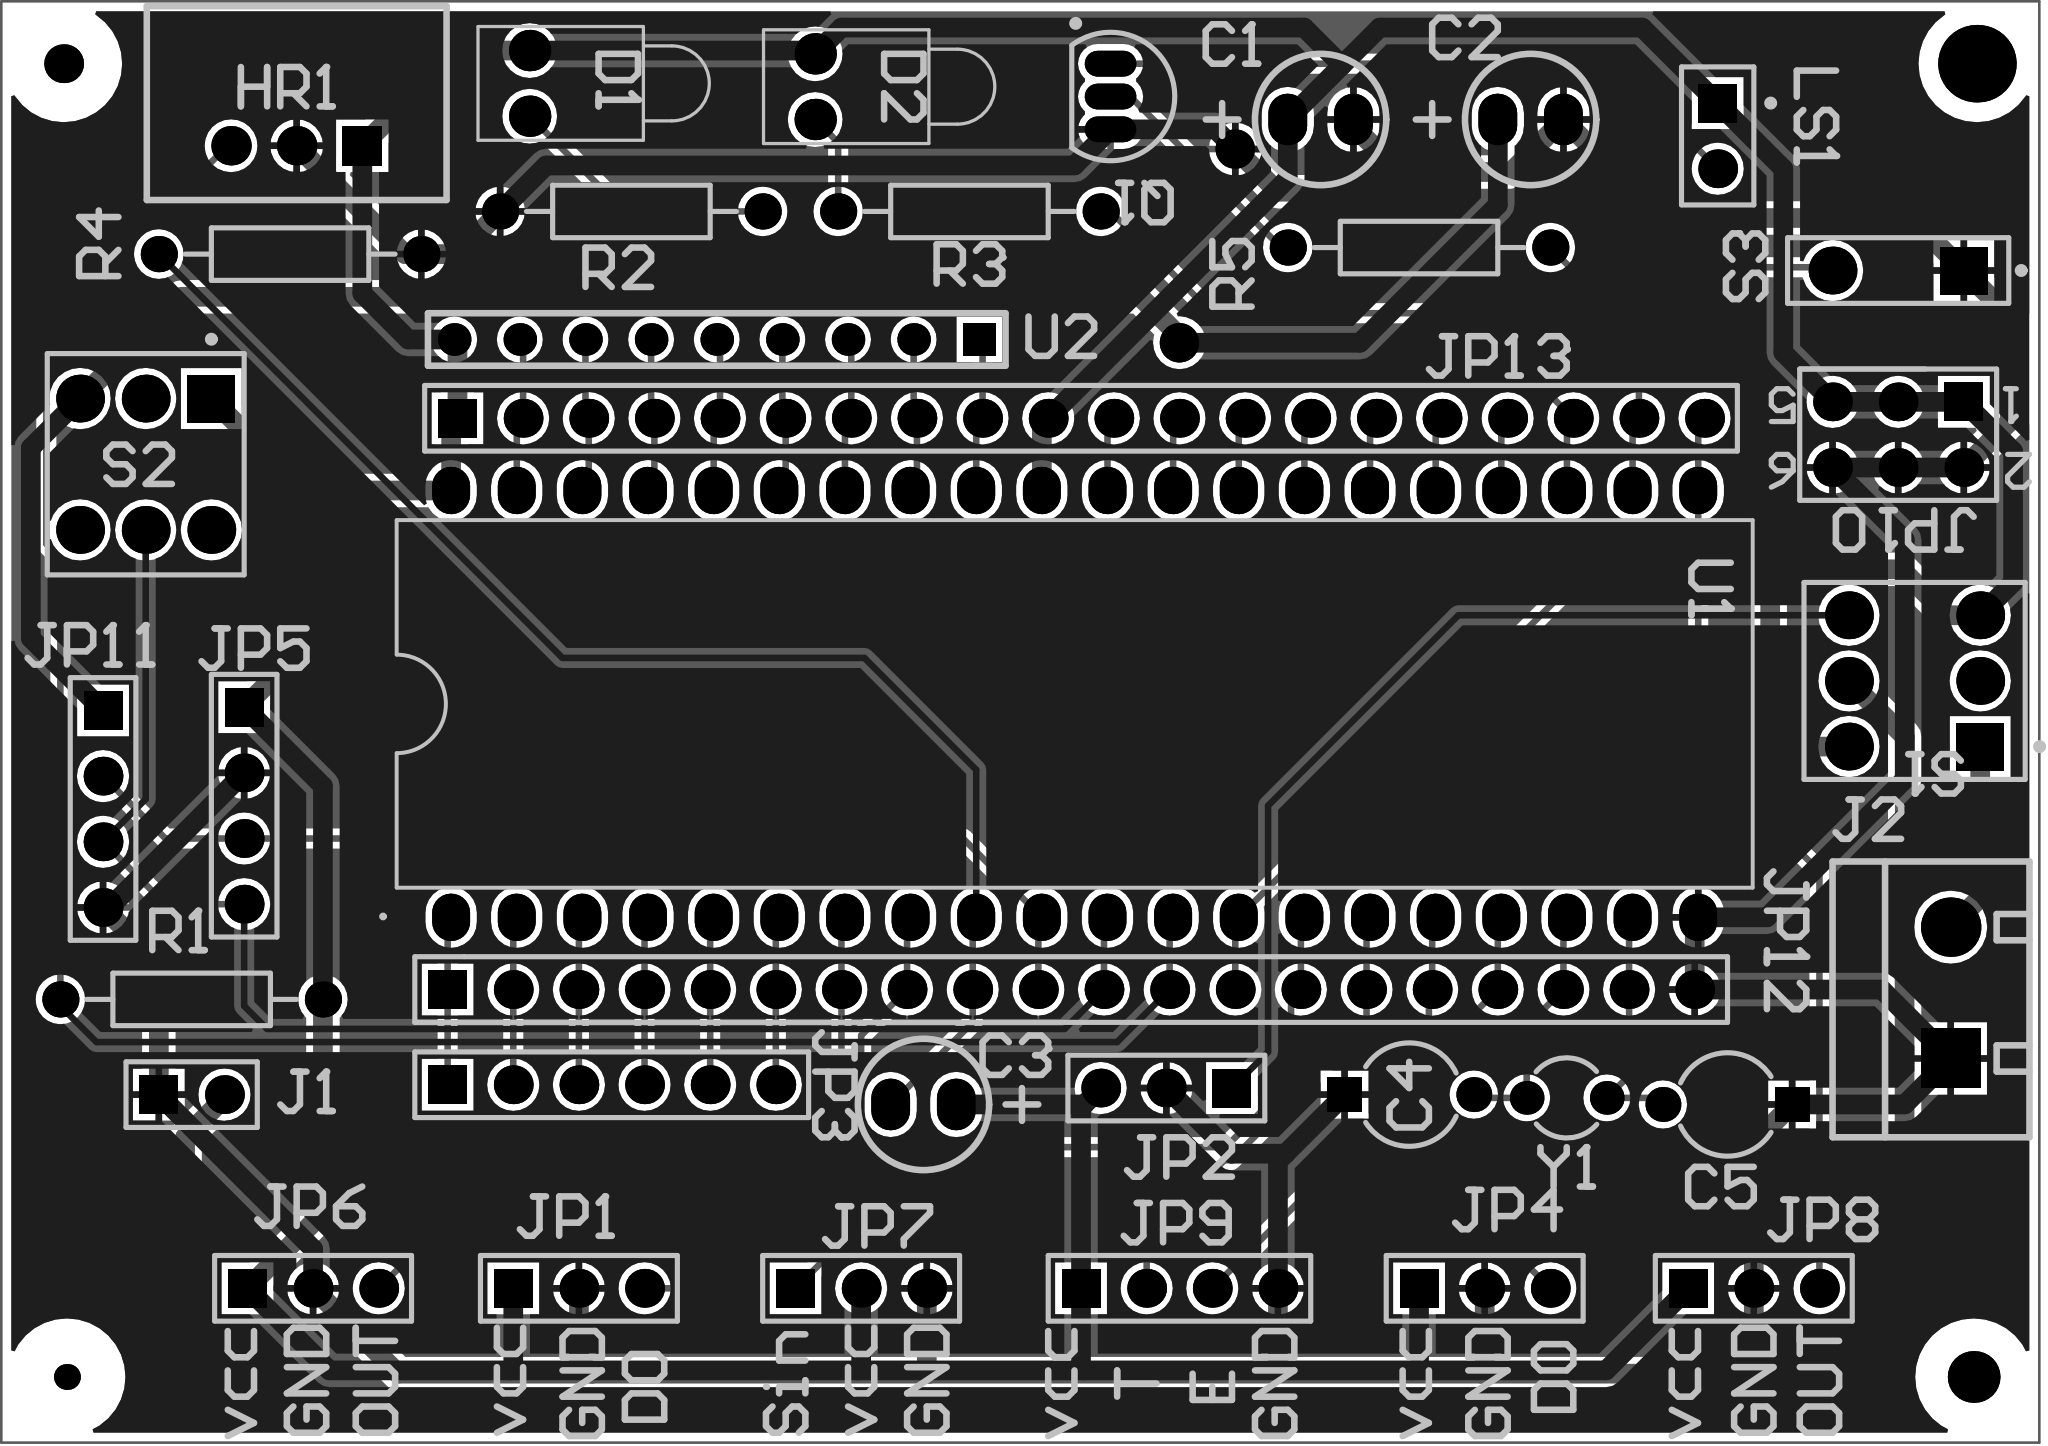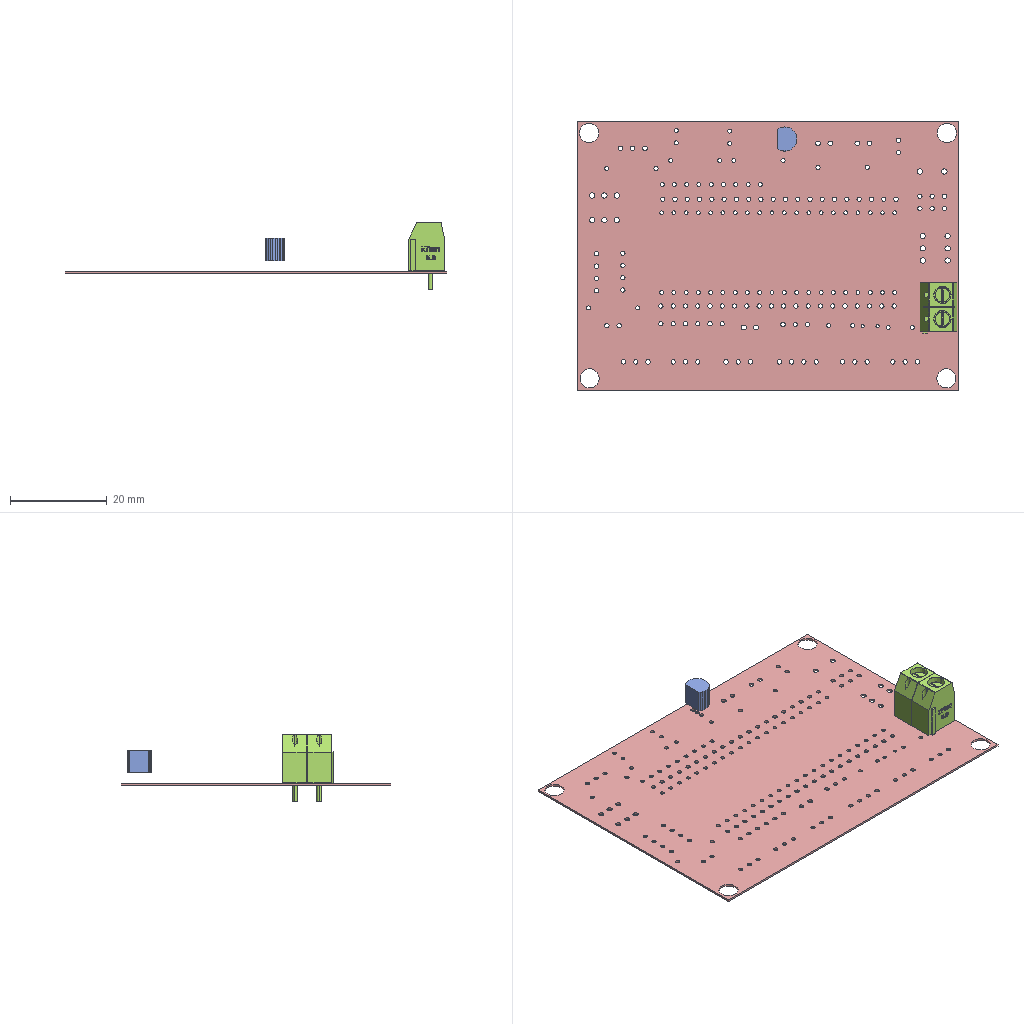Circuit board layout | Altium Designer | box 78.9 x 55.8 x 13.8 mm
Layer stack:
# Altium Designer layer stack of  (unit mm; dielectric type: 0 none, 1 core, 2 prepreg, 3 surface material)
index,name,kind,layer,copper_thickness_mm,dielectric_type,dielectric_thickness_mm,dielectric_material,dielectric_constant
0,Top Paste,other,,,,,,
1,Top Overlay,other,,,,,,
2,Top Solder,dielectric,,,3,0.0102,Solder Resist,3.5
3,Top Layer,copper,Top Layer,0.0356,,,,
4,Dielectric 1,dielectric,,,0,0.32,FR-4,4.8
5,Bottom Layer,copper,Bottom Layer,0.0356,,,,
6,Bottom Solder,dielectric,,,3,0.0102,Solder Resist,3.5
7,Bottom Overlay,other,,,,,,
8,Bottom Paste,other,,,,,,
# drill layer pairs: low layer,high layer
drill_pair,Top Layer,Bottom Layer
Part placement:
Designator,Comment,Layer,Footprint,Center-X(mm),Center-Y(mm),Rotation
Y1,11.059,TopLayer,R38,85.979,38.608,270
U2,Resistor network,TopLayer,paizu,53.086,67.945,180
U1,STC89C52RC,TopLayer,STC89C52RC,66.937,53.848,360
S3,SW-PB,TopLayer,SPST-2,98.806,70.612,180
S2,SW-DPDT,TopLayer,DPDT-6,30.988,63.119,270
S1,SW-DPDT,TopLayer,DPDT-6,99.441,54.737,180
R5,1K,TopLayer,AXIAL-0.4,80.264,71.501,180
R4,10K,TopLayer,AXIAL-0.4,36.576,71.247,180
R3,1K,TopLayer,AXIAL-0.4,62.865,72.898,360
R2,1K,TopLayer,AXIAL-0.4,49.784,72.898,180
R1,10K,TopLayer,AXIAL-0.4,32.766,42.418,180
Q1,2N3906,TopLayer,TO-92A,68.326,77.343,180
LS1,Bell,TopLayer,PIN2,91.821,75.819,270
JP13,Header 20,TopLayer,HDR1X20,67.183,64.897,360
JP12,Header 20,TopLayer,HDR1X20,66.802,42.799,360
JP11,Download interface,TopLayer,HDR1X4,29.337,49.784,270
JP10,Header 3X2,TopLayer,HDR2X3,98.806,64.262,180
JP9,Ultrasonic module,TopLayer,HDR1X4,70.993,31.242,360
JP8,Left obstacle avoidance,TopLayer,HDR1X3,93.218,31.242,360
JP7,Servo module,TopLayer,HDR1X3,58.674,31.242,360
JP6,Right obstacle avoidance,TopLayer,HDR1X3,37.465,31.242,360
JP5,Bluetooth module,TopLayer,HDR1X4,34.798,49.911,270
JP4,Left line tracking,TopLayer,HDR1X3,82.804,31.242,360
JP3,L298N control,TopLayer,HDR1X6,49.022,39.116,360
JP2,L298N power,TopLayer,HDR1X3,70.485,38.989,180
JP1,Right line tracking,TopLayer,HDR1X3,47.752,31.242,360
J2,KF301-2P,TopLayer,KF301-5.0-2P,100.838,42.672,90
J1,Header 2,TopLayer,HDR1X2,32.766,38.735,360
HR1,HR,TopLayer,SIP3,36.83,75.439,180
D2,Mode indicator LED,TopLayer,LED-1,56.896,77.724,360
D1,Power,TopLayer,LED-1,45.847,77.851,360
C5,22PF,TopLayer,CAPR5-4X5,92.202,38.354,180
C4,22PF,TopLayer,CAPR5-4X5,79.883,38.735,0
C3,10UF,TopLayer,DR,61.087,38.354,180
C2,470UF,TopLayer,DR,84.582,76.454,0
C1,470UF,TopLayer,DR,76.454,76.454,0
Pad and via stacks:
# Altium Designer via and pad stacks of  (unit mm). Each distinct definition once, with the count of objects using it.
# via: kind,start_layer,end_layer,hole_mm,diameter_mm,mode(0 simple;1 top-mid-bottom;2 full stack),diameter_per_layer,count,example_net
# pad: kind,layer,hole_mm,hole_type(0 round;1 square;2 slot),plating,top_size,top_shape(1 round;2 rect;3 octagon;9 rounded rect),mid_size,bottom_size,mode,footprint,size_per_layer,count,example
pad,Multi-Layer,4,0,plated,1.5x1.5,1,1.5x1.5,1.5x1.5,0,,,1,3
pad,Multi-Layer,4,0,plated,1x1,1,1x1,1x1,0,,,1,2
pad,Multi-Layer,4,0,plated,2x2,1,2x2,2x2,0,,,1,1
pad,Multi-Layer,4,0,plated,3x3,1,3x3,3x3,0,,,1,0
pad,Multi-Layer,0.9,0,plated,1.5x1.5,1,1.5x1.5,1.5x1.5,0,HDR1X4,,9,JP5.4
pad,Multi-Layer,0.9,0,plated,1.5x1.5,2,1.5x1.5,1.5x1.5,0,HDR1X4,,3,JP5.1
pad,Multi-Layer,1,0,plated,1.5x2,1,1.5x2,1.5x2,0,DR,,6,C3.1
pad,Multi-Layer,1.1,0,plated,1.85x1.85,1,1.85x1.85,1.85x1.85,0,DPDT-6,,10,S2.4
pad,Multi-Layer,1.1,0,plated,1.85x1.85,2,1.85x1.85,1.85x1.85,0,DPDT-6,,2,S2.1
pad,Multi-Layer,0.9,0,plated,1.5x1.5,2,1.5x1.5,1.5x1.5,0,HDR1X2,,1,J1.1
pad,Multi-Layer,0.9,0,plated,1.5x1.5,1,1.5x1.5,1.5x1.5,0,HDR1X2,,1,J1.2
pad,Multi-Layer,0.9144,0,plated,1.524x1.524,1,1.524x1.524,1.524x1.524,0,SIP3,,2,HR1.3
pad,Multi-Layer,0.9144,0,plated,1.524x1.524,2,1.524x1.524,1.524x1.524,0,SIP3,,1,HR1.1
pad,Multi-Layer,0.9,0,plated,1.5x1.5,2,1.5x1.5,1.5x1.5,0,HDR1X3,,6,JP1.1
pad,Multi-Layer,0.9,0,plated,1.5x1.5,1,1.5x1.5,1.5x1.5,0,HDR1X3,,12,JP1.2
pad,Multi-Layer,0.85,0,plated,1.4x1.4,1,1.4x1.4,1.4x1.4,0,AXIAL-0.4,,10,R1.1
pad,Multi-Layer,0.9,0,plated,1.5x1.5,2,1.5x1.5,1.5x1.5,0,HDR1X6,,1,JP3.1
pad,Multi-Layer,0.9,0,plated,1.5x1.5,1,1.5x1.5,1.5x1.5,0,HDR1X6,,5,JP3.2
pad,Multi-Layer,1.2,0,plated,2.3x2.3,2,2.3x2.3,2.3x2.3,0,KF301-5.0-2P,,1,J2.1
pad,Multi-Layer,1.2,0,plated,2.3x2.3,1,2.3x2.3,2.3x2.3,0,KF301-5.0-2P,,1,J2.2
pad,Multi-Layer,0.9,0,plated,1.5x1.5,2,1.5x1.5,1.5x1.5,0,HDR2X3,,1,JP10.1
pad,Multi-Layer,0.9,0,plated,1.5x1.5,1,1.5x1.5,1.5x1.5,0,HDR2X3,,5,JP10.2
pad,Multi-Layer,0.8,0,plated,1.6x1.6,1,1.6x1.6,1.6x1.6,0,LED-1,,4,D1.1
pad,Multi-Layer,0.9,0,plated,1.5x1.5,2,1.5x1.5,1.5x1.5,0,HDR1X20,,2,JP13.1
pad,Multi-Layer,0.9,0,plated,1.5x1.5,1,1.5x1.5,1.5x1.5,0,HDR1X20,,38,JP13.2
pad,Multi-Layer,0.84,0,plated,1.26x1.26,2,1.26x1.26,1.26x1.26,0,paizu,,1,U2.1
pad,Multi-Layer,0.84,0,plated,1.26x1.26,1,1.26x1.26,1.26x1.26,0,paizu,,8,U2.2
pad,Multi-Layer,0.8,0,plated,1.467x1.833,1,1.467x1.833,1.467x1.833,0,STC89C52RC,,40,U1.21
pad,Multi-Layer,1.1,0,plated,1.85x1.85,2,1.85x1.85,1.85x1.85,0,SPST-2,,1,S3.1
pad,Multi-Layer,1.1,0,plated,1.85x1.85,1,1.85x1.85,1.85x1.85,0,SPST-2,,1,S3.2
pad,Multi-Layer,0.9,0,plated,1.5x1.5,2,1.5x1.5,1.5x1.5,0,PIN2,,1,LS1.1
pad,Multi-Layer,0.9,0,plated,1.5x1.5,1,1.5x1.5,1.5x1.5,0,PIN2,,1,LS1.2
pad,Multi-Layer,0.8,0,plated,1.35x1.35,1,1.35x1.35,1.35x1.35,0,CAPR5-4X5,,2,C4.2
pad,Multi-Layer,0.8,0,plated,1.35x1.35,2,1.35x1.35,1.35x1.35,0,CAPR5-4X5,,2,C4.1
pad,Multi-Layer,0.7,0,plated,1.3x1.3,1,1.3x1.3,1.3x1.3,0,R38,,2,Y1.1
pad,Multi-Layer,0.9,0,plated,2x1,1,2x1,2x1,0,TO-92A,,3,Q1.3
via,Top Layer,Bottom Layer,0.762,1.524,0,,2,GND
Copper pours:
name,layer,net,type(0 solid;1 hatched;2 none)
Top Layer-No Net,Bottom Layer,GND,0
Top Layer-No Net,Top Layer,GND,0
Design rules, without the lines most boards share:
# Altium Designer design rules of  (exported by Altium Designer, unit mm)
# columns: name | kind | enabled | priority | scope1 | scope2 | descriptor | typed fields (field=value)
SilkToSilkClearance | 55 | enabled | 1 | All | All | Silk to Silk (Clearance=0mil) (All),(All) |
SilkToSolderMaskClearance | 54 | enabled | 1 | IsPad | All | Silk To Solder Mask (Clearance=0mil) (IsPad),(All) |
MinimumSolderMaskSliver | 53 | enabled | 1 | All | All | Minimum Solder Mask Sliver (Gap=0mil) (All),(All) |
HoleToHoleClearance | 52 | enabled | 1 | All | All | Hole To Hole Clearance (Gap=10mil) (All),(All) | gap=0.254
DiffPairsRouting | 51 | enabled | 1 | All | All | Differential Pairs Uncoupled Length using the Gap Constraints (Min=10mil) (Max=10mil) (Prefered=10mil)  and Width Constraints (Min=15mil) (Max=15mil) (Prefered=15mil) (All) |
SolderMaskExpansion | 13 | enabled | 1 | All | All | Solder Mask Expansion (Expansion =4mil) (All) | expansion=0.1016
PasteMaskExpansion | 14 | enabled | 1 | All | All | Paste Mask Expansion (Expansion =0mil) (All) | expansion=0
RoutingVias | 11 | enabled | 1 | All | All | Routing Via (MinHoleWidth=28mil) (MaxHoleWidth=28mil) (PreferredHoleWidth=28mil) (MinWidth=50mil) (MaxWidth=50mil) (PreferedWidth=50mil) (All) | via_min_hole=0.7112 via_max_hole=0.7112 via_preferred_diameter=1.27 via_preferred_hole=0.7112
Width | 2 | enabled | 1 | All | All | Width Constraint (Min=10mil) (Max=30mil) (Preferred=10mil) (All) |
PolygonConnect | 20 | enabled | 1 | All | All | Polygon Connect Rule(Relief Connect )(Conductor Width=10mil) (Relief Angle=90 Angle) (Entries=4) (Air Gap Width=10mil) (All),(All) | connect_style(0=relief,1=direct,2=none)=0 relief_conductor_width=0.254 relief_entries=4
PlaneConnect | 6 | enabled | 1 | All | All | Power Plane Connect Rule(Relief Connect )(Expansion=20mil) (Conductor Width=10mil) (Air Gap=10mil) (Entries=4) (All) | relief_conductor_width=0.254 relief_entries=4 relief_expansion=0.508
Clearance | 0 | enabled | 1 | All | All | Clearance Constraint (Gap=10mil) (All),(All) | gap=0.254
Classes set for this board:
# Altium Designer classes of  (member kind: 0 net, 1 component, 2 from-to, 3 pad, 4 layer, 5 differential pair, 6 design channel, 7 polygon, 8 structure, 9 xSignal)
# columns: class name | member kind | superclass | members
Sheet1 | 1 | no | C1; C2; C3; C4; C5; D1; D2; HR1; J1; J2; JP1; JP2; JP3; JP4; JP5; JP6; JP7; JP8; JP9; JP10; JP11; JP12; JP13; LS1; Q1; R1; R2; R3; R4; R5; S1; S2; S3; U1; U2; Y1;